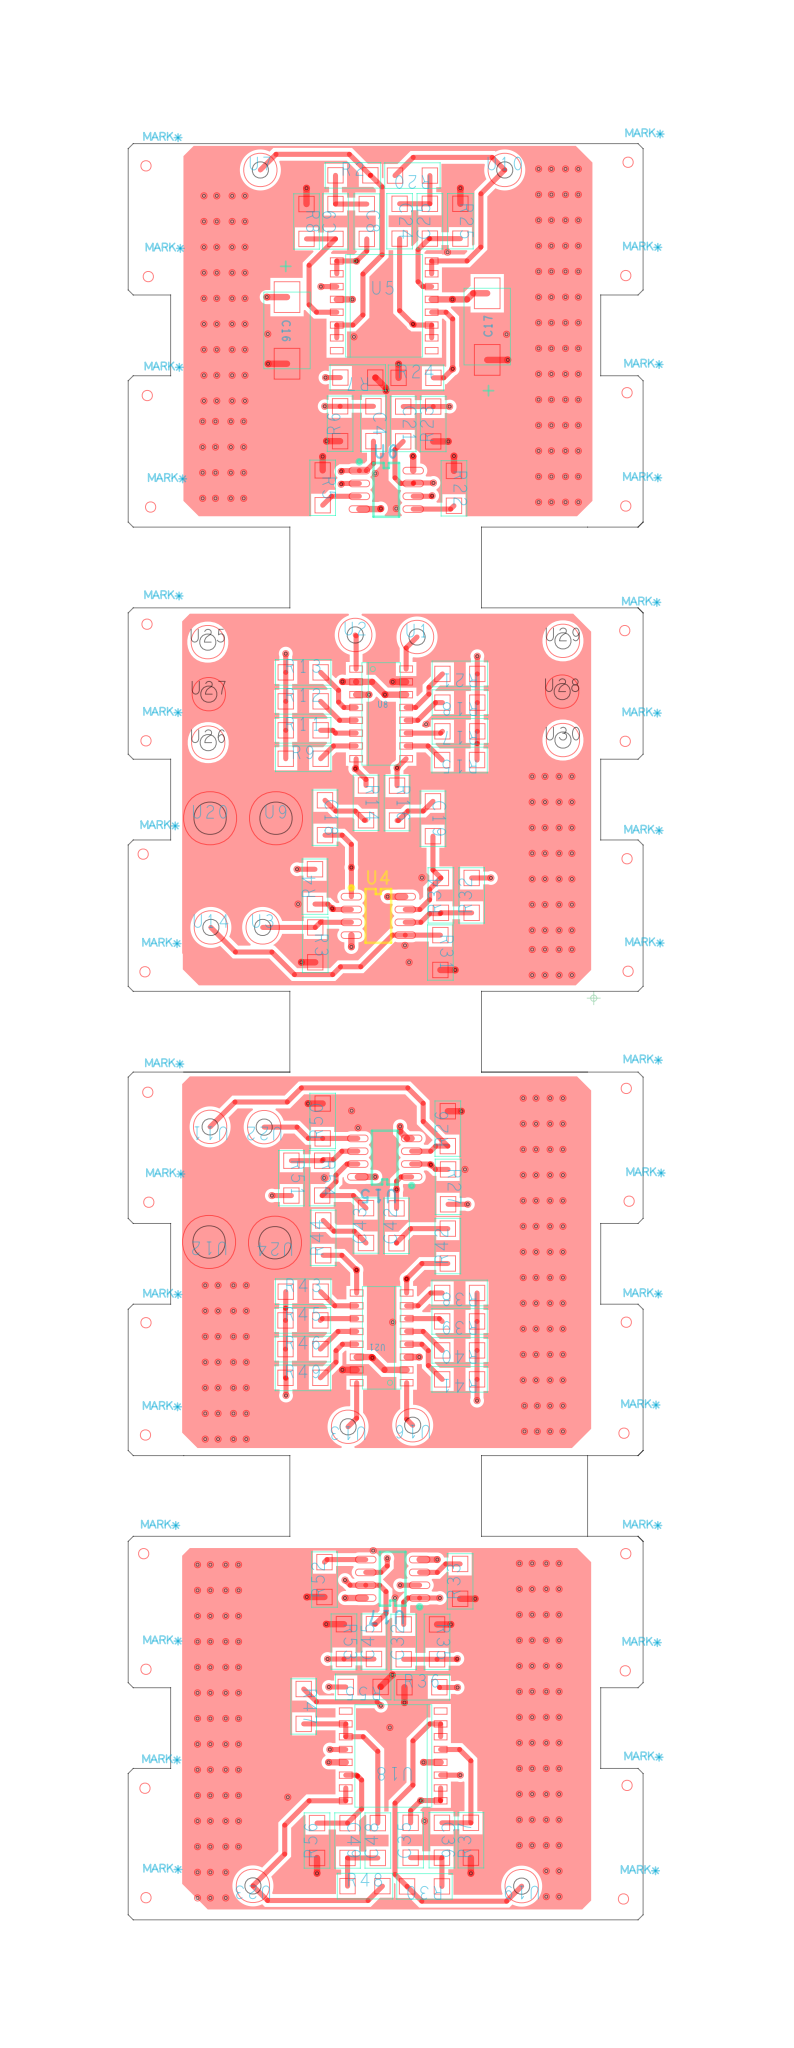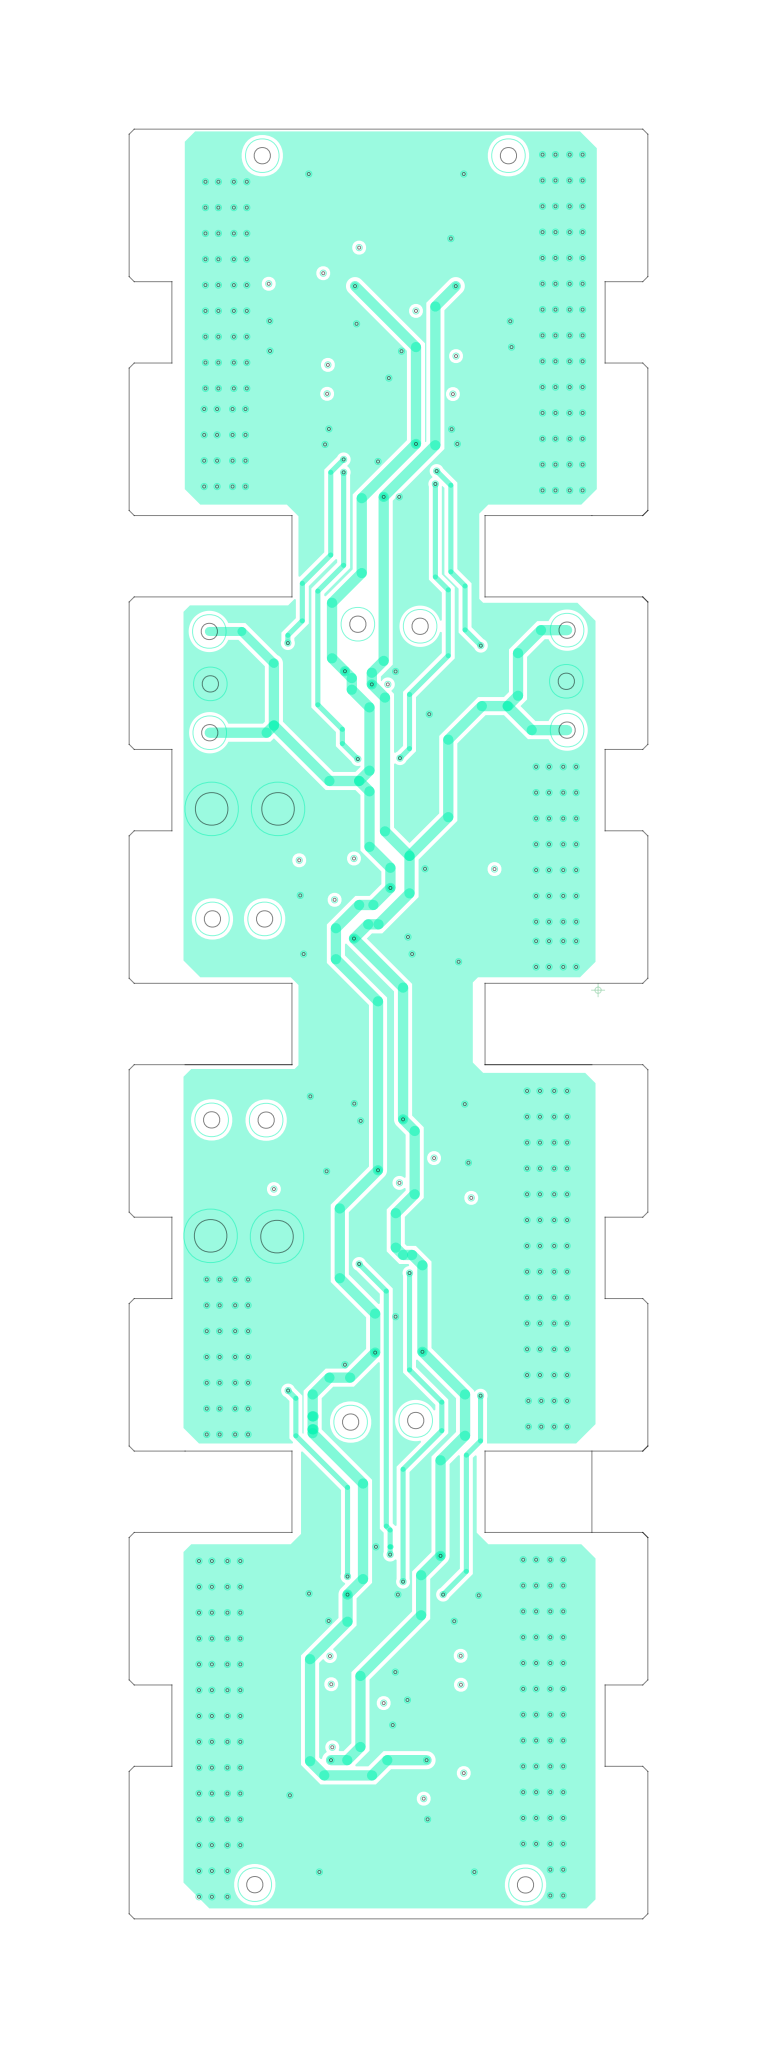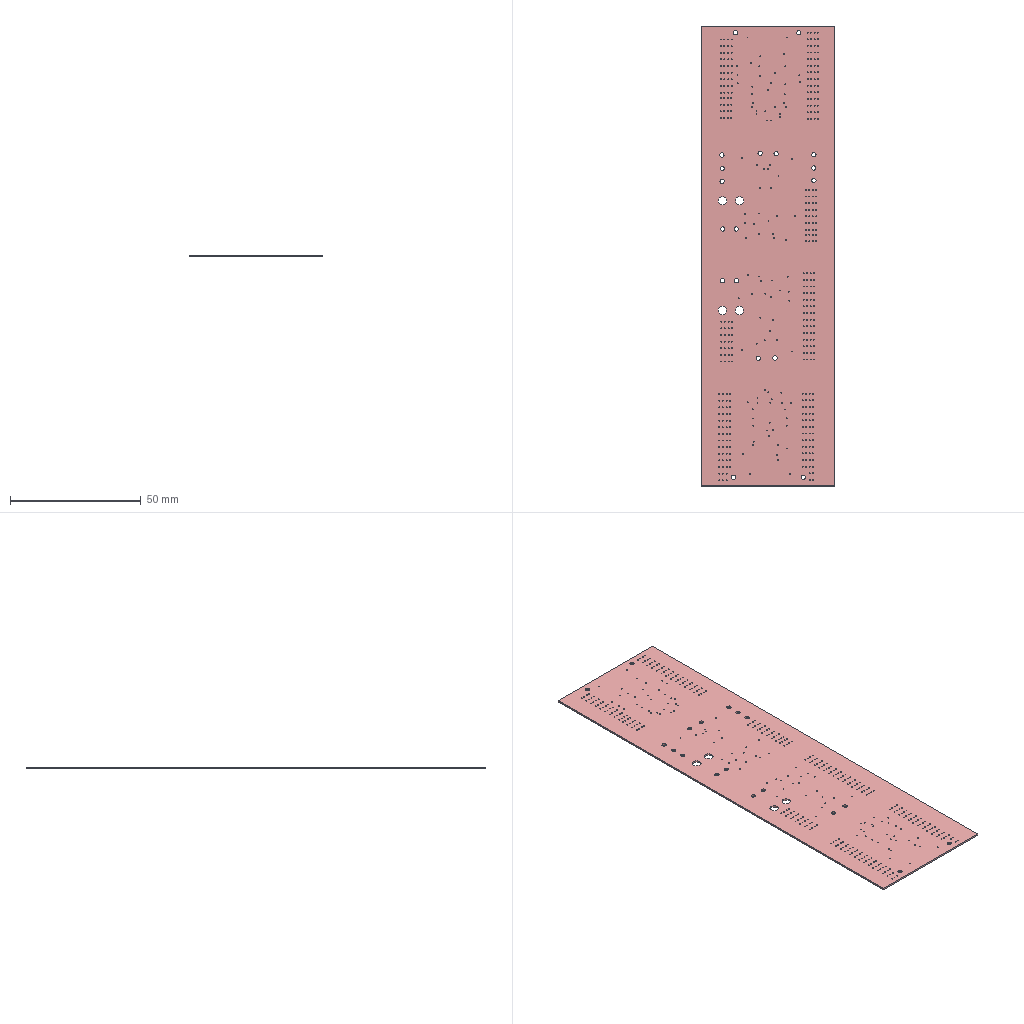Circuit board layout | Cadence Allegro | box 51 x 176 x 0.7 mm
Layer stack:
# Cadence Allegro layer stack of  (unit mm; from the constraint file cross-section; dielectric type: 0 not recorded (Allegro does not mark core vs prepreg), 3 surface material)
index,name,kind,layer,copper_thickness_mm,dielectric_type,dielectric_thickness_mm,dielectric_material,dielectric_constant
0,Top Surface,other,,,,,,
1,TOP,copper,TOP,0.0305,,,,
2,Dielectric1,dielectric,,,0,0.2032,FR-4,4.5
3,SIG2,copper,SIG2,0.0305,,,,
4,Dielectric2,dielectric,,,0,0.2032,FR-4,4.5
5,SIG3,copper,SIG3,0.0305,,,,
6,Dielectric3,dielectric,,,0,0.2032,FR-4,4.5
7,BOTTOM,copper,BOTTOM,0.0305,,,,
8,Bottom Surface,other,,,,,,
# drill layer pairs: low layer,high layer
drill_pair,TOP,BOTTOM
Part placement:
REFDES,COMP_VALUE,SYM_NAME,SYM_X,SYM_Y,SYM_ROTATE,SYM_MIRROR
C1,0.1uF,1206,-736,330,90.000,YES
C2,0.1uF,1206,-707,1992,270.000,YES
C3,0.1uF,1206,-630,2815,90.000,YES
C4,100nF,1206,-859,2241,270.000,NO
C5,100nF,1206,-919,2299,0.000,YES
C6,0.1uF,1206,-848,140,180.000,YES
C7,100nF,1206,-920,2421,180.000,YES
C8,100nF,1206,-885,3030,270.000,NO
C9,100nF,1206,-1007,3030,90.000,NO
C10,0.047uF,1206,-1087,435,90.000,YES
C11,0.1uF,1206,-915,1979,90.000,YES
C12,0.1uF,1206,-994,2648,270.000,YES
C13,0.01uF,1206,-735,1119,270.000,YES
C14,0.01uF,1206,-1196,2659,270.000,YES
C15,0.01uF,1206,-417,2658,270.000,YES
C16,10uF/50V,7343,-1196,2605,270.000,NO
C17,10uF/50V,7343,-415.35,2619.921,90.000,NO
C18,100nF,1206,-1048,704,270.000,NO
C19,100nF,1206,-627,700,270.000,NO
C20,0.1uF,1206,-928,1116,270.000,YES
C21,100nF,1206,-743,2240,270.000,NO
C22,100nF,1206,-692,2298,180.000,YES
C23,100nF,1206,-692,2419,0.000,YES
C24,100nF,1206,-757,3031,270.000,NO
C25,100nF,1206,-639,3031,90.000,NO
C26,0.047uF,1206,-568,-736,270.000,YES
C27,0.1uF,1206,-919,-631,270.000,YES
C28,0.1uF,1206,-730,-2913,90.000,YES
C29,0.1uF,1206,-822,-439,0.000,YES
C30,0.047uF,1206,-536,470,0.000,YES
C31,0.1uF,1206,-964,-3050,270.000,YES
C32,100nF,1206,-741,-2511,90.000,NO
C33,100nF,1206,-671,-2577,180.000,YES
C34,100nF,1206,-669,-2689,0.000,YES
C35,100nF,1206,-714,-3285,90.000,NO
C36,100nF,1206,-592,-3285,270.000,NO
C37,0.1uF,1206,-678,-2261,270.000,YES
C38,0.1uF,1206,-886,-2274,90.000,YES
C39,0.01uF,1206,-921,-1335,90.000,YES
C40,0.01uF,1206,-728,-3142,270.000,YES
C41,0.01uF,1206,-1135,-3049,270.000,YES
C42,100nF,1206,-769,-888,90.000,NO
C43,100nF,1206,-888,-887,90.000,NO
C44,0.1uF,1206,-728,-1332,90.000,YES
C45,100nF,1206,-857,-2510,90.000,NO
C46,100nF,1206,-898,-2577,0.000,YES
C47,100nF,1206,-898,-2687,180.000,YES
C48,100nF,1206,-842,-3286,90.000,NO
C49,100nF,1206,-960,-3286,270.000,NO
C50,0.047uF,1206,-1119,-771,180.000,YES
R1,1.21K,1206,-854,2646,270.000,YES
R2,1.21K,1206,-939,3210,0.000,NO
R3,2.4M,1206,-1086,208,270.000,NO
R4,13.6K,1206,-1087,435,90.000,NO
R5,3K,1206,-1057,1991,270.000,NO
R6,20K,1206,-989,2241,90.000,NO
R7,3.32K,1206,-920,2421,180.000,NO
R8,3.32K,1206,-1120,3030,270.000,NO
R9,60.4K,1206,-1133,934,0.000,NO
R10,13.6K,1206,-945,377,270.000,YES
R11,30K,1206,-1133,1045,0.000,NO
R12,15K,1206,-1133,1158,0.000,NO
R13,7.5K,1206,-1133,1271,0.000,NO
R14,3K,1206,-888,762,270.000,NO
R15,60.4K,1206,-523,929,180.000,NO
R16,3K,1206,-767,761,270.000,NO
R17,30K,1206,-522,1041,180.000,NO
R18,15K,1206,-522,1153,180.000,NO
R19,1.21K,1206,-629,2588,270.000,YES
R20,1.21K,1206,-707,3209,180.000,NO
R21,7.5K,1206,-522,1265,180.000,NO
R22,3K,1206,-545,1989,270.000,NO
R23,20K,1206,-626,2240,90.000,NO
R24,3.32K,1206,-693,2420,0.000,NO
R25,3.32K,1206,-520,3031,270.000,NO
R26,2.4M,1206,-569,-509,90.000,NO
R27,13.6K,1206,-568,-736,270.000,NO
R28,13.6K,1206,-710,-678,90.000,YES
R29,1.21K,1206,-595,-3006,90.000,YES
R30,1.21K,1206,-660,-3465,180.000,NO
R31,2.4M,1206,-598,178,270.000,NO
R32,13.6K,1206,-476,401,90.000,NO
R33,3K,1206,-521,-2275,90.000,NO
R34,13.6K,1206,-596,401,90.000,NO
R35,20K,1206,-611,-2511,270.000,NO
R36,3.32K,1206,-670,-2688,0.000,NO
R37,3.32K,1206,-479,-3285,90.000,NO
R38,60.4K,1206,-523,-1150,180.000,NO
R39,30K,1206,-523,-1261,180.000,NO
R40,15K,1206,-523,-1374,180.000,NO
R41,7.5K,1206,-523,-1487,180.000,NO
R42,3K,1206,-569,-967,90.000,NO
R43,60.4K,1206,-1133,-1145,0.000,NO
R44,3K,1206,-1055,-935,90.000,NO
R45,30K,1206,-1134,-1257,0.000,NO
R46,15K,1206,-1134,-1369,0.000,NO
R47,1.21K,1206,-1131,-2763,270.000,NO
R48,1.21K,1206,-892,-3464,0.000,NO
R49,7.5K,1206,-1134,-1481,0.000,NO
R50,2.4M,1206,-1057,-479,90.000,NO
R51,13.6K,1206,-1179,-702,270.000,NO
R52,3K,1206,-1050,-2268,90.000,NO
R53,20K,1206,-974,-2510,270.000,NO
R54,13.6K,1206,-1059,-702,270.000,NO
R55,3.32K,1206,-899,-2687,180.000,NO
R56,3.32K,1206,-1079,-3286,90.000,NO
U1,CONNECTP,CPAD80,-689,1409,0.000,NO
U2,CONNECTP,CPAD80,-930,1417,0.000,NO
U3,CONNECTP,CPAD80,-1291,276,0.000,NO
U4,op284,SO-8,-840,321,0.000,NO
U5,OP470,SOIC16W,-817,2701,0.000,NO
U6,op824,SO-8,-809,1983,0.000,NO
U7,CONNECTP,CPAD80,-1300,3231,0.000,NO
U8,ADG406,SO-16,-829,1109,0.000,NO
U9,CONNECTP,DP250CIR,-1239,702,0.000,NO
U10,CONNECTP,CPAD80,-347,3231,0.000,NO
U11,CONNECTP,CPAD80,-1496,-502,180.000,NO
U12,CONNECTP,DP250CIR,-1500,-951,180.000,NO
U13,CONNECTP,CPAD80,-958,-1672,180.000,NO
U14,CONNECTP,CPAD80,-1493,276,0.000,NO
U15,op284,SO-8,-815,-622,180.000,NO
U16,CONNECTP,CPAD80,-706,-1666,180.000,NO
U17,op824,SO-8,-784,-2265,180.000,NO
U18,OP470,SOIC16W,-782,-2956,180.000,NO
U19,CONNECTP,CPAD80,-281,-3464,180.000,NO
U20,CONNECTP,DP250CIR,-1496,702,0.000,NO
U21,ADG406,SO-16,-827,-1325,180.000,NO
U22,CONNECTP,CPAD80,-1285,-503,180.000,NO
U23,CONNECTP,CPAD80,-1329,-3463,180.000,NO
U24,CONNECTP,DP250CIR,-1243,-954,180.000,NO
U25,CONNECTP,CPAD80,-1505,1389,0.000,NO
U26,CONNECTP,CPAD80,-1503.35,996.921,0.000,NO
U27,CONNECTP,CPAD80,-1501,1186,0.000,NO
U28,CONNECTP,CPAD80,-123,1196,0.000,NO
U29,CONNECTP,CPAD80,-120,1394,0.000,NO
U30,CONNECTP,CPAD80,-120,1007,0.000,NO
Pad and via stacks:
# Allegro (Cadence) via spans and padstacks; design units: ("mils" 4 10000)
# via spans: padstack,start_layer,end_layer,net_example,count
VIA12_24,ETCH/TOP,ETCH/BOTTOM,AGND,436
# Allegro padstack definitions: name,start_layer,end_layer,drill,plating,holeType,type
SMDSQR_60,"ETCH/TOP","ETCH/TOP",0.0,"PLATED","none","smd"
R120X1001,"ETCH/TOP","ETCH/TOP",0.0,"PLATED","none","smd"
SMT080X026,"ETCH/TOP","ETCH/TOP",0.0,"PLATED","none","smd"
SMD50_25,"ETCH/TOP","ETCH/TOP",0.0,"PLATED","none","smd"
MARKPOINT,"ETCH/TOP","ETCH/TOP",0.0,"PLATED","none","smd"
VIA_24D12,"ETCH/TOP","ETCH/BOTTOM",12.0,"PLATED","circle_drill","through"
VIA_20D10,"ETCH/TOP","ETCH/BOTTOM",10.0,"PLATED","circle_drill","through"
VIA_U,"ETCH/TOP","ETCH/BOTTOM",25.0,"PLATED","circle_drill","through"
VIA,"ETCH/TOP","ETCH/BOTTOM",13.0,"PLATED","circle_drill","through"
PAD-C207D126,"ETCH/TOP","ETCH/BOTTOM",126.0,"PLATED","circle_drill","through"
HOLE88,"ETCH/TOP","ETCH/BOTTOM",63.0,"PLATED","circle_drill","through"
VIA12_24,"ETCH/TOP","ETCH/BOTTOM",12.0,"PLATED","circle_drill","through"
Design rules, without the lines most boards share, first 14 of 27 lines:
# Cadence Allegro design rules of  (from the Constraint Manager export constraints.dcfx, design unit mil; typed fields in mm)
# columns: name | kind | enabled | priority | scope1 | scope2 | descriptor | typed fields (field=value)
# Allegro precedence (priority 1 wins): 1 Region class-to-class, 2 Region class, 3 Region, 4 class-to-class, 5 DiffPair/Bus/NetGroup override, 6 NetClass, 7 constraint set (CSet) default
# per-layer values are written LAYER=value in the descriptor and LAYER:mm in the typed field; a maximum of 0 means no limit set
# --- net classes (and buses / net groups) ---
# (no net classes defined: every net uses the default constraint sets)
# --- track widths, neck and differential-pair gap (physical constraint sets) ---
DEFAULT | PhysicalCSet | enabled | 7 | Design default | All | Physical Constraint (Min Line Width=10mil) (Max Line Width=50mil) (Min Neck Width=8mil) (Max Neck Length=1000mil) (DiffPair Primary Gap=0mil) (DiffPair Neck Gap=0mil) (DiffPair Min Space=0mil) (DiffPair Coupled +Tol=0mil) (DiffPair Coupled -Tol=0mil) (Min BB Via Stagger=5mil) (Max BB Via Stagger=0mil) (T-junctions=ANYWHERE) (Pad-pad direct connect=ALL_ALLOWED) (Allowed vias=VIA12_24, VIA_20D10, VIA_24D12) | min_line_width=0.254 min_neck_width=0.2032 min_bvia_stagger=0.127 max_bvia_stagger=0 ts_allowed=ANYWHERE diffp_primary_gap=0 diffp_neck_gap=0 max_line_width=1.27 maximum_neck_length=25.4 pad_pad_direct_connect=ALL_ALLOWED allow_on_etch_subclass=TRUE diffp_coupled_plus=0 diffp_coupled_minus=0 diffp_min_space=0 vias=VIA12_24,VIA_20D10,VIA_24D12
PWR | PhysicalCSet | enabled | 7 | not referenced | All | Physical Constraint (Min Line Width=20mil) (Max Line Width=50mil) (Min Neck Width=8mil) (Max Neck Length=1000mil) (DiffPair Primary Gap=0mil) (DiffPair Neck Gap=0mil) (DiffPair Min Space=0mil) (DiffPair Coupled +Tol=0mil) (DiffPair Coupled -Tol=0mil) (Min BB Via Stagger=5mil) (Max BB Via Stagger=0mil) (T-junctions=ANYWHERE) (Pad-pad direct connect=ALL_ALLOWED) (Allowed vias=VIA_24D12, VIA_20D10) | min_line_width=0.508 min_neck_width=0.2032 min_bvia_stagger=0.127 max_bvia_stagger=0 ts_allowed=ANYWHERE diffp_primary_gap=0 diffp_neck_gap=0 max_line_width=1.27 maximum_neck_length=25.4 pad_pad_direct_connect=ALL_ALLOWED allow_on_etch_subclass=TRUE diffp_coupled_plus=0 diffp_coupled_minus=0 diffp_min_space=0 vias=VIA_24D12,VIA_20D10
# --- clearances: line / pad / via / shape / hole (spacing constraint sets) ---
DEFAULT | SpacingCSet | enabled | 7 | Design default | All | Clearance Constraint (Line-Line=8mil) (Line-SMD Pad=8mil) (Line-Thru Pin=8mil) (Line-Via=8mil) (Line-Shape=15mil) (SMD Pad-SMD Pad=8mil) (Thru Pin-Thru Pin=8mil) (Thru Pin-SMD Pad=8mil) (SMD Pad-Via=8mil) (Thru Pin-Via=8mil) (Via-Via=8mil) (Shape-SMD Pad=15mil) (Shape-Thru Pin=15mil) (Shape-Via=15mil) (Shape-Shape=15mil) (Hole-Hole=5mil) (Hole-Line=8mil) (Hole-Shape=15mil) (BB Via-BB Via=8mil) (uVia-uVia=8mil) | thrupin_to_thrupin_spacing=0.2032 thrupin_to_smdpin_spacing=0.2032 thrupin_to_thruvia_spacing=0.2032 line_to_thrupin_spacing=0.2032 thrupin_to_shape_spacing=0.381 smdpin_to_smdpin_spacing=0.2032 smdpin_to_thruvia_spacing=0.2032 line_to_smdpin_spacing=0.2032 shape_to_smdpin_spacing=0.381 thruvia_to_thruvia_spacing=0.2032 line_to_thruvia_spacing=0.2032 shape_to_thruvia_spacing=0.381 line_to_line_spacing=0.2032 line_to_shape_spacing=0.381 shape_to_shape_spacing=0.381 bbv_to_bbv_spacing=0.2032 bbv_to_thrupin_spacing=0.2032 bbv_to_smdpin_spacing=0.2032 bbv_to_thruvia_spacing=0.2032 bbv_to_line_spacing=0.2032 bbv_to_shape_spacing=0.381 bbv_to_testpin_spacing=0.2032 bbv_to_testvia_spacing=0.2032 testpin_to_testpin_spacing=0.2032 testpin_to_thrupin_spacing=0.2032 smdpin_to_testpin_spacing=0.2032 testpin_to_thruvia_spacing=0.2032 testpin_to_testvia_spacing=0.2032 line_to_testpin_spacing=0.2032 shape_to_testpin_spacing=0.381 testvia_to_testvia_spacing=0.2032 testvia_to_thrupin_spacing=0.2032 smdpin_to_testvia_spacing=0.2032 testvia_to_thruvia_spacing=0.2032 line_to_testvia_spacing=0.2032 shape_to_testvia_spacing=0.381 bondpad_to_bondpad_spacing=0.127 thrupin_to_bondpad_spacing=0.2032 smdpin_to_bondpad_spacing=0.2032 bondpad_to_thruvia_spacing=0.2032 bondpad_to_line_spacing=0.2032 bondpad_to_shape_spacing=0.381 bondpad_to_bbv_spacing=0.2032 bondpad_to_testpin_spacing=0.2032 bondpad_to_testvia_spacing=0.2032 min_bvia_gap=0.127 hole_to_pin_spacing=0.2032 hole_to_via_spacing=0.2032 hole_to_line_spacing=0.2032 hole_to_shape_spacing=0.381 hole_to_hole_spacing=0.127 mvia_to_mvia_spacing=0.2032 mvia_to_thrupin_spacing=0.2032 mvia_to_smdpin_spacing=0.2032 mvia_to_thruvia_spacing=0.2032 mvia_to_bbv_spacing=0.2032 mvia_to_line_spacing=0.2032 mvia_to_shape_spacing=0.381 mvia_to_testpin_spacing=0.2032 mvia_to_testvia_spacing=0.2032 bondpad_to_mvia_spacing=0.2032 bondpad_to_bondpad_diffp_spc=0.127
DEFAULT | SameNetSpacingCSet | enabled | 7 | Design default | All | Same-Net Clearance (Line-Line=8mil) (Line-SMD Pad=7mil) (Line-Thru Pin=8mil) (Line-Via=8mil) (Line-Shape=8mil) (SMD Pad-SMD Pad=6mil) (Thru Pin-Thru Pin=8mil) (Thru Pin-SMD Pad=8mil) (SMD Pad-Via=5mil) (Thru Pin-Via=5mil) (Via-Via=5mil) (Shape-SMD Pad=5mil) (Shape-Thru Pin=5mil) (Shape-Via=5mil) (Shape-Shape=5mil) (Hole-Hole=5mil) (Hole-Line=5mil) (Hole-Shape=5mil) (BB Via-BB Via=5mil) (uVia-uVia=5mil) | sn_thrupin_to_thrupin_spacing=0.2032 sn_thrupin_to_smdpin_spacing=0.2032 sn_thrupin_to_thruvia_spacing=0.127 sn_line_to_thrupin_spacing=0.2032 sn_thrupin_to_shape_spacing=0.127 sn_smdpin_to_smdpin_spacing=0.1524 sn_smdpin_to_thruvia_spacing=0.127 sn_line_to_smdpin_spacing=0.1778 sn_shape_to_smdpin_spacing=0.127 sn_thruvia_to_thruvia_spacing=0.127 sn_line_to_thruvia_spacing=0.2032 sn_shape_to_thruvia_spacing=0.127 sn_line_to_line_spacing=0.2032 sn_line_to_shape_spacing=0.2032 sn_shape_to_shape_spacing=0.127 sn_bbv_to_bbv_spacing=0.127 sn_bbv_to_thrupin_spacing=0.127 sn_bbv_to_smdpin_spacing=0.127 sn_bbv_to_thruvia_spacing=0.127 sn_bbv_to_line_spacing=0.2032 sn_bbv_to_shape_spacing=0.127 sn_bbv_to_testpin_spacing=0.127 sn_bbv_to_testvia_spacing=0.127 sn_testpin_to_testpin_spacing=8 sn_testpin_to_thrupin_spacing=0.2032 sn_smdpin_to_testpin_spacing=0.2032 sn_testpin_to_thruvia_spacing=0.127 sn_testpin_to_testvia_spacing=0.127 sn_line_to_testpin_spacing=0.2032 sn_shape_to_testpin_spacing=0.127 sn_testvia_to_testvia_spacing=0.127 sn_testvia_to_thrupin_spacing=0.127 sn_smdpin_to_testvia_spacing=0.127 sn_testvia_to_thruvia_spacing=0.127 sn_line_to_testvia_spacing=0.2032 sn_shape_to_testvia_spacing=0.127 sn_bondpad_to_bondpad_spacing=0.127 sn_thrupin_to_bondpad_spacing=0.127 sn_smdpin_to_bondpad_spacing=0.127 sn_bondpad_to_thruvia_spacing=0.127 sn_bondpad_to_line_spacing=0.2032 sn_bondpad_to_shape_spacing=0.127 sn_bondpad_to_bbv_spacing=0.127 sn_bondpad_to_testpin_spacing=0.127 sn_bondpad_to_testvia_spacing=0.127 same_net=TRUE sn_hole_to_pin_spacing=0.127 sn_hole_to_via_spacing=0.127 sn_hole_to_line_spacing=0.127 sn_hole_to_shape_spacing=0.127 sn_hole_to_hole_spacing=0.127 sn_mvia_to_mvia_spacing=0.127 sn_mvia_to_thrupin_spacing=0.127 sn_mvia_to_smdpin_spacing=0.127 sn_mvia_to_thruvia_spacing=0.127 sn_mvia_to_bbv_spacing=0.127 sn_mvia_to_line_spacing=0.2032 sn_mvia_to_shape_spacing=0.127 sn_mvia_to_testpin_spacing=0.127 sn_mvia_to_testvia_spacing=0.127 sn_bondpad_to_mvia_spacing=0.127
# --- differential pairs (0) ---
# (no differential pairs defined)